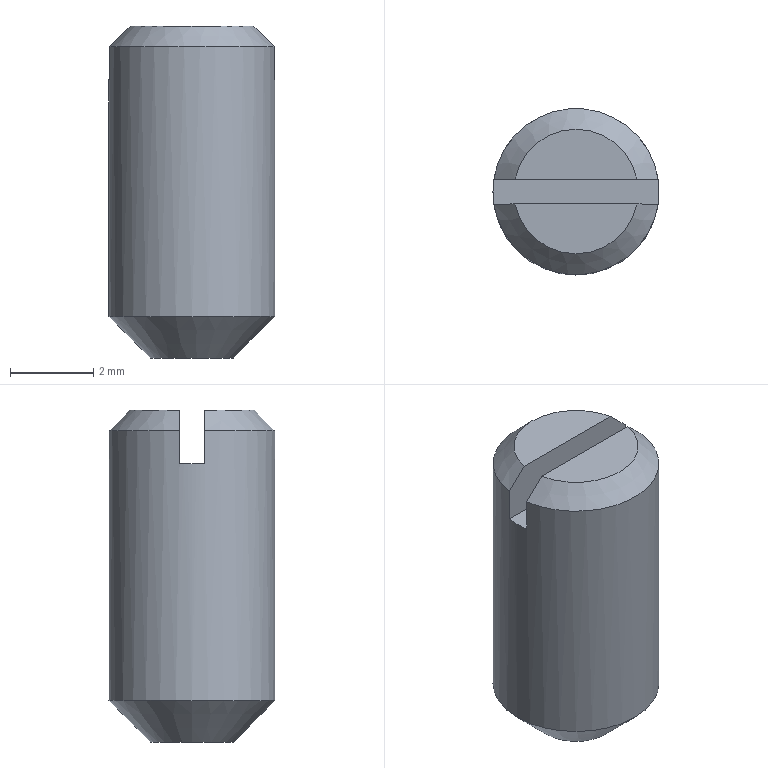Part | NX | features DATUM_CSYS 3, CHAMFER 2, SKETCH 2, EXTRUDE 1, SWP104 1, SYMBOLIC_THREAD 1 | 1 solid | 10 faces | box 4 x 4 x 8 mm | volume 90.888 mm3 | plane 6 | cone 3 | cylinder 1 | commonest cylinder face diameters 4 x1
STEP:
#1=CARTESIAN_POINT('',(-1.47,-0.3,8.));
#2=VERTEX_POINT('',#1);
#3=CARTESIAN_POINT('',(1.47,-0.3,8.));
#4=VERTEX_POINT('',#3);
#5=CARTESIAN_POINT('',(-3.7,-0.3,8.));
#6=DIRECTION('',(1.,0.,0.));
#7=VECTOR('',#6,1000.);
#8=LINE('',#5,#7);
#9=EDGE_CURVE('',#2,#4,#8,.T.);
#10=ORIENTED_EDGE('',*,*,#9,.F.);
#11=CARTESIAN_POINT('',(0.,0.,8.));
#12=DIRECTION('',(0.,0.,1.));
#13=DIRECTION('',(1.,0.,0.));
#14=AXIS2_PLACEMENT_3D('',#11,#12,#13);
#15=CIRCLE('',#14,1.5);
#16=EDGE_CURVE('',#2,#4,#15,.T.);
#17=ORIENTED_EDGE('',*,*,#16,.T.);
#18=EDGE_LOOP('',(#10,#17));
#19=FACE_BOUND('',#18,.T.);
#20=CARTESIAN_POINT('',(0.,2.,8.));
#21=DIRECTION('',(0.,0.,1.));
#22=DIRECTION('',(1.,0.,0.));
#23=AXIS2_PLACEMENT_3D('',#20,#21,#22);
#24=PLANE('',#23);
#25=ADVANCED_FACE('',(#19),#24,.T.);
#26=CARTESIAN_POINT('',(-1.977,-0.3,7.5));
#27=VERTEX_POINT('',#26);
#28=CARTESIAN_POINT('',(-1.977,-0.3,7.5));
#29=CARTESIAN_POINT('',(-1.808,-0.3,7.667));
#30=CARTESIAN_POINT('',(-1.639,-0.3,7.834));
#31=CARTESIAN_POINT('',(-1.47,-0.3,8.));
#32=B_SPLINE_CURVE_WITH_KNOTS('',3,(#28,#29,#30,#31),.UNSPECIFIED.,.F.,.F.,(4,4),(0.00343,0.004142),.UNSPECIFIED.);
#33=EDGE_CURVE('',#27,#2,#32,.T.);
#34=ORIENTED_EDGE('',*,*,#33,.F.);
#35=CARTESIAN_POINT('',(1.977,-0.3,7.5));
#36=VERTEX_POINT('',#35);
#37=CARTESIAN_POINT('',(0.,0.,7.5));
#38=DIRECTION('',(0.,0.,1.));
#39=DIRECTION('',(1.,0.,0.));
#40=AXIS2_PLACEMENT_3D('',#37,#38,#39);
#41=CIRCLE('',#40,2.);
#42=EDGE_CURVE('',#36,#27,#41,.F.);
#43=ORIENTED_EDGE('',*,*,#42,.F.);
#44=CARTESIAN_POINT('',(1.47,-0.3,8.));
#45=CARTESIAN_POINT('',(1.639,-0.3,7.834));
#46=CARTESIAN_POINT('',(1.808,-0.3,7.667));
#47=CARTESIAN_POINT('',(1.977,-0.3,7.5));
#48=B_SPLINE_CURVE_WITH_KNOTS('',3,(#44,#45,#46,#47),.UNSPECIFIED.,.F.,.F.,(4,4),(0.007997,0.008716),.UNSPECIFIED.);
#49=EDGE_CURVE('',#4,#36,#48,.T.);
#50=ORIENTED_EDGE('',*,*,#49,.F.);
#51=ORIENTED_EDGE('',*,*,#16,.F.);
#52=EDGE_LOOP('',(#34,#43,#50,#51));
#53=FACE_BOUND('',#52,.T.);
#54=CARTESIAN_POINT('',(0.,0.,7.5));
#55=DIRECTION('',(0.,0.,-1.));
#56=DIRECTION('',(-1.,0.,0.));
#57=AXIS2_PLACEMENT_3D('',#54,#55,#56);
#58=CONICAL_SURFACE('',#57,2.,0.7854);
#59=ADVANCED_FACE('',(#53),#58,.T.);
#60=CARTESIAN_POINT('',(-1.,0.,0.));
#61=VERTEX_POINT('',#60);
#62=CARTESIAN_POINT('',(0.,0.,0.));
#63=DIRECTION('',(0.,0.,-1.));
#64=DIRECTION('',(-1.,0.,0.));
#65=AXIS2_PLACEMENT_3D('',#62,#63,#64);
#66=CIRCLE('',#65,1.);
#67=EDGE_CURVE('',#61,#61,#66,.T.);
#68=ORIENTED_EDGE('',*,*,#67,.T.);
#69=EDGE_LOOP('',(#68));
#70=FACE_BOUND('',#69,.T.);
#71=CARTESIAN_POINT('',(0.,0.,0.));
#72=DIRECTION('',(0.,0.,-1.));
#73=DIRECTION('',(-1.,0.,0.));
#74=AXIS2_PLACEMENT_3D('',#71,#72,#73);
#75=PLANE('',#74);
#76=ADVANCED_FACE('',(#70),#75,.T.);
#77=CARTESIAN_POINT('',(-1.977,-0.3,6.7));
#78=VERTEX_POINT('',#77);
#79=CARTESIAN_POINT('',(-1.977,-0.3,0.));
#80=DIRECTION('',(0.,0.,-1.));
#81=VECTOR('',#80,1000.);
#82=LINE('',#79,#81);
#83=EDGE_CURVE('',#78,#27,#82,.F.);
#84=ORIENTED_EDGE('',*,*,#83,.F.);
#85=CARTESIAN_POINT('',(-1.977,0.3,6.7));
#86=VERTEX_POINT('',#85);
#87=CARTESIAN_POINT('',(0.,0.,6.7));
#88=DIRECTION('',(0.,0.,1.));
#89=DIRECTION('',(1.,0.,0.));
#90=AXIS2_PLACEMENT_3D('',#87,#88,#89);
#91=CIRCLE('',#90,2.);
#92=EDGE_CURVE('',#78,#86,#91,.F.);
#93=ORIENTED_EDGE('',*,*,#92,.T.);
#94=CARTESIAN_POINT('',(-1.977,0.3,7.5));
#95=VERTEX_POINT('',#94);
#96=CARTESIAN_POINT('',(-1.977,0.3,0.));
#97=DIRECTION('',(0.,0.,-1.));
#98=VECTOR('',#97,1000.);
#99=LINE('',#96,#98);
#100=EDGE_CURVE('',#95,#86,#99,.T.);
#101=ORIENTED_EDGE('',*,*,#100,.F.);
#102=CARTESIAN_POINT('',(1.977,0.3,7.5));
#103=VERTEX_POINT('',#102);
#104=CARTESIAN_POINT('',(0.,0.,7.5));
#105=DIRECTION('',(0.,0.,1.));
#106=DIRECTION('',(1.,0.,0.));
#107=AXIS2_PLACEMENT_3D('',#104,#105,#106);
#108=CIRCLE('',#107,2.);
#109=EDGE_CURVE('',#95,#103,#108,.F.);
#110=ORIENTED_EDGE('',*,*,#109,.T.);
#111=CARTESIAN_POINT('',(1.977,0.3,6.7));
#112=VERTEX_POINT('',#111);
#113=CARTESIAN_POINT('',(1.977,0.3,0.));
#114=DIRECTION('',(0.,0.,-1.));
#115=VECTOR('',#114,1000.);
#116=LINE('',#113,#115);
#117=EDGE_CURVE('',#112,#103,#116,.F.);
#118=ORIENTED_EDGE('',*,*,#117,.F.);
#119=CARTESIAN_POINT('',(1.977,-0.3,6.7));
#120=VERTEX_POINT('',#119);
#121=CARTESIAN_POINT('',(0.,0.,6.7));
#122=DIRECTION('',(0.,0.,1.));
#123=DIRECTION('',(1.,0.,0.));
#124=AXIS2_PLACEMENT_3D('',#121,#122,#123);
#125=CIRCLE('',#124,2.);
#126=EDGE_CURVE('',#112,#120,#125,.F.);
#127=ORIENTED_EDGE('',*,*,#126,.T.);
#128=CARTESIAN_POINT('',(1.977,-0.3,0.));
#129=DIRECTION('',(0.,0.,-1.));
#130=VECTOR('',#129,1000.);
#131=LINE('',#128,#130);
#132=EDGE_CURVE('',#36,#120,#131,.T.);
#133=ORIENTED_EDGE('',*,*,#132,.F.);
#134=ORIENTED_EDGE('',*,*,#42,.T.);
#135=EDGE_LOOP('',(#84,#93,#101,#110,#118,#127,#133,#134));
#136=FACE_BOUND('',#135,.T.);
#137=CARTESIAN_POINT('',(-2.,0.,1.));
#138=VERTEX_POINT('',#137);
#139=CARTESIAN_POINT('',(0.,0.,1.));
#140=DIRECTION('',(0.,0.,-1.));
#141=DIRECTION('',(-1.,0.,0.));
#142=AXIS2_PLACEMENT_3D('',#139,#140,#141);
#143=CIRCLE('',#142,2.);
#144=EDGE_CURVE('',#138,#138,#143,.F.);
#145=ORIENTED_EDGE('',*,*,#144,.T.);
#146=EDGE_LOOP('',(#145));
#147=FACE_BOUND('',#146,.T.);
#148=CARTESIAN_POINT('',(0.,0.,0.));
#149=DIRECTION('',(0.,0.,-1.));
#150=DIRECTION('',(-1.,0.,0.));
#151=AXIS2_PLACEMENT_3D('',#148,#149,#150);
#152=CYLINDRICAL_SURFACE('',#151,2.);
#153=ADVANCED_FACE('',(#136,#147),#152,.T.);
#154=CARTESIAN_POINT('',(1.47,0.3,8.));
#155=VERTEX_POINT('',#154);
#156=CARTESIAN_POINT('',(-1.47,0.3,8.));
#157=VERTEX_POINT('',#156);
#158=CARTESIAN_POINT('',(3.7,0.3,8.));
#159=DIRECTION('',(-1.,0.,0.));
#160=VECTOR('',#159,1000.);
#161=LINE('',#158,#160);
#162=EDGE_CURVE('',#155,#157,#161,.T.);
#163=ORIENTED_EDGE('',*,*,#162,.F.);
#164=CARTESIAN_POINT('',(0.,0.,8.));
#165=DIRECTION('',(0.,0.,1.));
#166=DIRECTION('',(1.,0.,0.));
#167=AXIS2_PLACEMENT_3D('',#164,#165,#166);
#168=CIRCLE('',#167,1.5);
#169=EDGE_CURVE('',#155,#157,#168,.T.);
#170=ORIENTED_EDGE('',*,*,#169,.T.);
#171=EDGE_LOOP('',(#163,#170));
#172=FACE_BOUND('',#171,.T.);
#173=CARTESIAN_POINT('',(0.,2.,8.));
#174=DIRECTION('',(0.,0.,1.));
#175=DIRECTION('',(1.,0.,0.));
#176=AXIS2_PLACEMENT_3D('',#173,#174,#175);
#177=PLANE('',#176);
#178=ADVANCED_FACE('',(#172),#177,.T.);
#179=CARTESIAN_POINT('',(1.977,0.3,7.5));
#180=CARTESIAN_POINT('',(1.808,0.3,7.667));
#181=CARTESIAN_POINT('',(1.639,0.3,7.834));
#182=CARTESIAN_POINT('',(1.47,0.3,8.));
#183=B_SPLINE_CURVE_WITH_KNOTS('',3,(#179,#180,#181,#182),.UNSPECIFIED.,.F.,.F.,(4,4),(0.00343,0.004142),.UNSPECIFIED.);
#184=EDGE_CURVE('',#103,#155,#183,.T.);
#185=ORIENTED_EDGE('',*,*,#184,.F.);
#186=ORIENTED_EDGE('',*,*,#109,.F.);
#187=CARTESIAN_POINT('',(-1.47,0.3,8.));
#188=CARTESIAN_POINT('',(-1.639,0.3,7.834));
#189=CARTESIAN_POINT('',(-1.808,0.3,7.667));
#190=CARTESIAN_POINT('',(-1.977,0.3,7.5));
#191=B_SPLINE_CURVE_WITH_KNOTS('',3,(#187,#188,#189,#190),.UNSPECIFIED.,.F.,.F.,(4,4),(0.007997,0.008716),.UNSPECIFIED.);
#192=EDGE_CURVE('',#157,#95,#191,.T.);
#193=ORIENTED_EDGE('',*,*,#192,.F.);
#194=ORIENTED_EDGE('',*,*,#169,.F.);
#195=EDGE_LOOP('',(#185,#186,#193,#194));
#196=FACE_BOUND('',#195,.T.);
#197=CARTESIAN_POINT('',(0.,0.,7.5));
#198=DIRECTION('',(0.,0.,-1.));
#199=DIRECTION('',(-1.,0.,0.));
#200=AXIS2_PLACEMENT_3D('',#197,#198,#199);
#201=CONICAL_SURFACE('',#200,2.,0.7854);
#202=ADVANCED_FACE('',(#196),#201,.T.);
#203=ORIENTED_EDGE('',*,*,#144,.F.);
#204=EDGE_LOOP('',(#203));
#205=FACE_BOUND('',#204,.T.);
#206=ORIENTED_EDGE('',*,*,#67,.F.);
#207=EDGE_LOOP('',(#206));
#208=FACE_BOUND('',#207,.T.);
#209=CARTESIAN_POINT('',(0.,0.,0.));
#210=DIRECTION('',(0.,0.,1.));
#211=DIRECTION('',(1.,0.,0.));
#212=AXIS2_PLACEMENT_3D('',#209,#210,#211);
#213=CONICAL_SURFACE('',#212,1.,0.7854);
#214=ADVANCED_FACE('',(#205,#208),#213,.T.);
#215=ORIENTED_EDGE('',*,*,#83,.T.);
#216=ORIENTED_EDGE('',*,*,#33,.T.);
#217=ORIENTED_EDGE('',*,*,#9,.T.);
#218=ORIENTED_EDGE('',*,*,#49,.T.);
#219=ORIENTED_EDGE('',*,*,#132,.T.);
#220=CARTESIAN_POINT('',(-3.7,-0.3,6.7));
#221=DIRECTION('',(1.,0.,0.));
#222=VECTOR('',#221,1000.);
#223=LINE('',#220,#222);
#224=EDGE_CURVE('',#120,#78,#223,.F.);
#225=ORIENTED_EDGE('',*,*,#224,.T.);
#226=EDGE_LOOP('',(#215,#216,#217,#218,#219,#225));
#227=FACE_BOUND('',#226,.T.);
#228=CARTESIAN_POINT('',(-3.7,-0.3,6.7));
#229=DIRECTION('',(0.,-1.,0.));
#230=DIRECTION('',(0.,0.,-1.));
#231=AXIS2_PLACEMENT_3D('',#228,#229,#230);
#232=PLANE('',#231);
#233=ADVANCED_FACE('',(#227),#232,.F.);
#234=ORIENTED_EDGE('',*,*,#117,.T.);
#235=ORIENTED_EDGE('',*,*,#184,.T.);
#236=ORIENTED_EDGE('',*,*,#162,.T.);
#237=ORIENTED_EDGE('',*,*,#192,.T.);
#238=ORIENTED_EDGE('',*,*,#100,.T.);
#239=CARTESIAN_POINT('',(3.7,0.3,6.7));
#240=DIRECTION('',(-1.,0.,0.));
#241=VECTOR('',#240,1000.);
#242=LINE('',#239,#241);
#243=EDGE_CURVE('',#86,#112,#242,.F.);
#244=ORIENTED_EDGE('',*,*,#243,.T.);
#245=EDGE_LOOP('',(#234,#235,#236,#237,#238,#244));
#246=FACE_BOUND('',#245,.T.);
#247=CARTESIAN_POINT('',(3.7,0.3,6.7));
#248=DIRECTION('',(0.,1.,0.));
#249=DIRECTION('',(0.,0.,1.));
#250=AXIS2_PLACEMENT_3D('',#247,#248,#249);
#251=PLANE('',#250);
#252=ADVANCED_FACE('',(#246),#251,.F.);
#253=ORIENTED_EDGE('',*,*,#224,.F.);
#254=ORIENTED_EDGE('',*,*,#126,.F.);
#255=ORIENTED_EDGE('',*,*,#243,.F.);
#256=ORIENTED_EDGE('',*,*,#92,.F.);
#257=EDGE_LOOP('',(#253,#254,#255,#256));
#258=FACE_BOUND('',#257,.T.);
#259=CARTESIAN_POINT('',(0.,0.,6.7));
#260=DIRECTION('',(0.,0.,1.));
#261=DIRECTION('',(1.,0.,0.));
#262=AXIS2_PLACEMENT_3D('',#259,#260,#261);
#263=PLANE('',#262);
#264=ADVANCED_FACE('',(#258),#263,.T.);
#265=CLOSED_SHELL('',(#25,#59,#76,#153,#178,#202,#214,#233,#252,#264));
#266=MANIFOLD_SOLID_BREP('',#265);
#267=(LENGTH_UNIT()NAMED_UNIT(*)SI_UNIT(.MILLI.,.METRE.));
#268=UNCERTAINTY_MEASURE_WITH_UNIT(LENGTH_MEASURE(0.0508),#267,'','');
#269=(NAMED_UNIT(*)PLANE_ANGLE_UNIT()SI_UNIT($,.RADIAN.));
#270=(NAMED_UNIT(*)SI_UNIT($,.STERADIAN.)SOLID_ANGLE_UNIT());
#271=(GEOMETRIC_REPRESENTATION_CONTEXT(3)GLOBAL_UNCERTAINTY_ASSIGNED_CONTEXT((#268))GLOBAL_UNIT_ASSIGNED_CONTEXT((#267,#269,#270))REPRESENTATION_CONTEXT('',''));
#272=ADVANCED_BREP_SHAPE_REPRESENTATION('',(#266),#271);